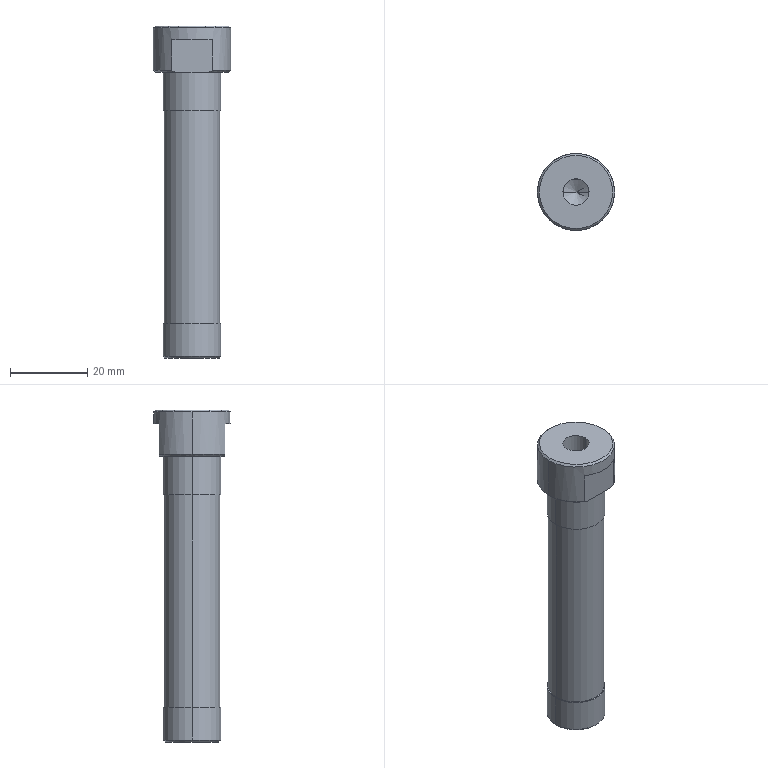Part | STEP file | 10000020474swp000-1 | 1 solid | 32 faces | box 20 x 20 x 86 mm | volume 15036 mm3 | cylinder 12 | cone 11 | plane 9 | commonest cylinder face diameters 15 x4 3.3 x2 6.8 x2 14.4 x2 20 x2
STEP:
#1=CARTESIAN_POINT('',(1.65,0.,-73.9));
#2=VERTEX_POINT('',#1);
#3=CARTESIAN_POINT('',(-1.65,0.,-73.9));
#4=VERTEX_POINT('',#3);
#5=CARTESIAN_POINT('',(0.,0.,-73.9));
#6=DIRECTION('',(0.,0.,-1.));
#7=DIRECTION('',(-1.,0.,0.));
#8=AXIS2_PLACEMENT_3D('',#5,#6,#7);
#9=CIRCLE('',#8,1.65);
#10=EDGE_CURVE('',#2,#4,#9,.T.);
#11=ORIENTED_EDGE('',*,*,#10,.F.);
#12=CARTESIAN_POINT('',(1.65,0.,-86.));
#13=VERTEX_POINT('',#12);
#14=CARTESIAN_POINT('',(1.65,0.,-86.));
#15=DIRECTION('',(0.,0.,-1.));
#16=VECTOR('',#15,1000.);
#17=LINE('',#14,#16);
#18=EDGE_CURVE('',#2,#13,#17,.T.);
#19=ORIENTED_EDGE('',*,*,#18,.T.);
#20=CARTESIAN_POINT('',(-1.65,0.,-86.));
#21=VERTEX_POINT('',#20);
#22=CARTESIAN_POINT('',(0.,0.,-86.));
#23=DIRECTION('',(0.,0.,-1.));
#24=DIRECTION('',(-1.,0.,0.));
#25=AXIS2_PLACEMENT_3D('',#22,#23,#24);
#26=CIRCLE('',#25,1.65);
#27=EDGE_CURVE('',#13,#21,#26,.T.);
#28=ORIENTED_EDGE('',*,*,#27,.T.);
#29=CARTESIAN_POINT('',(-1.65,0.,-86.));
#30=DIRECTION('',(0.,0.,-1.));
#31=VECTOR('',#30,1000.);
#32=LINE('',#29,#31);
#33=EDGE_CURVE('',#4,#21,#32,.T.);
#34=ORIENTED_EDGE('',*,*,#33,.F.);
#35=EDGE_LOOP('',(#11,#19,#28,#34));
#36=FACE_OUTER_BOUND('',#35,.T.);
#37=CARTESIAN_POINT('',(0.,0.,-86.));
#38=DIRECTION('',(0.,0.,-1.));
#39=DIRECTION('',(-1.,0.,0.));
#40=AXIS2_PLACEMENT_3D('',#37,#38,#39);
#41=CYLINDRICAL_SURFACE('',#40,1.65);
#42=ADVANCED_FACE('',(#36),#41,.F.);
#43=CARTESIAN_POINT('',(0.,0.,-72.909));
#44=VERTEX_POINT('',#43);
#45=CARTESIAN_POINT('',(-1.65,0.,-73.9));
#46=DIRECTION('',(-0.8572,0.,-0.515));
#47=VECTOR('',#46,1000.);
#48=LINE('',#45,#47);
#49=EDGE_CURVE('',#44,#4,#48,.T.);
#50=ORIENTED_EDGE('',*,*,#49,.F.);
#51=CARTESIAN_POINT('',(1.65,0.,-73.9));
#52=DIRECTION('',(0.8572,0.,-0.515));
#53=VECTOR('',#52,1000.);
#54=LINE('',#51,#53);
#55=EDGE_CURVE('',#44,#2,#54,.T.);
#56=ORIENTED_EDGE('',*,*,#55,.T.);
#57=ORIENTED_EDGE('',*,*,#10,.T.);
#58=EDGE_LOOP('',(#50,#56,#57));
#59=FACE_OUTER_BOUND('',#58,.T.);
#60=CARTESIAN_POINT('',(0.,0.,-73.9));
#61=DIRECTION('',(0.,0.,-1.));
#62=DIRECTION('',(-1.,0.,0.));
#63=AXIS2_PLACEMENT_3D('',#60,#61,#62);
#64=CONICAL_SURFACE('',#63,1.65,1.03);
#65=ADVANCED_FACE('',(#59),#64,.F.);
#66=CARTESIAN_POINT('',(9.5,0.,0.));
#67=VERTEX_POINT('',#66);
#68=CARTESIAN_POINT('',(-9.5,0.,0.));
#69=VERTEX_POINT('',#68);
#70=CARTESIAN_POINT('',(0.,0.,0.));
#71=DIRECTION('',(0.,0.,1.));
#72=DIRECTION('',(1.,0.,0.));
#73=AXIS2_PLACEMENT_3D('',#70,#71,#72);
#74=CIRCLE('',#73,9.5);
#75=EDGE_CURVE('',#67,#69,#74,.T.);
#76=ORIENTED_EDGE('',*,*,#75,.F.);
#77=CARTESIAN_POINT('',(10.,0.,-0.5));
#78=VERTEX_POINT('',#77);
#79=CARTESIAN_POINT('',(9.5,0.,0.));
#80=DIRECTION('',(0.7071,0.,-0.7071));
#81=VECTOR('',#80,1000.);
#82=LINE('',#79,#81);
#83=EDGE_CURVE('',#67,#78,#82,.T.);
#84=ORIENTED_EDGE('',*,*,#83,.T.);
#85=CARTESIAN_POINT('',(-10.,0.,-0.5));
#86=VERTEX_POINT('',#85);
#87=CARTESIAN_POINT('',(0.,0.,-0.5));
#88=DIRECTION('',(0.,0.,-1.));
#89=DIRECTION('',(1.,0.,0.));
#90=AXIS2_PLACEMENT_3D('',#87,#88,#89);
#91=CIRCLE('',#90,10.);
#92=EDGE_CURVE('',#86,#78,#91,.T.);
#93=ORIENTED_EDGE('',*,*,#92,.F.);
#94=CARTESIAN_POINT('',(-9.5,0.,0.));
#95=DIRECTION('',(-0.7071,0.,-0.7071));
#96=VECTOR('',#95,1000.);
#97=LINE('',#94,#96);
#98=EDGE_CURVE('',#69,#86,#97,.T.);
#99=ORIENTED_EDGE('',*,*,#98,.F.);
#100=EDGE_LOOP('',(#76,#84,#93,#99));
#101=FACE_OUTER_BOUND('',#100,.T.);
#102=CARTESIAN_POINT('',(0.,0.,0.));
#103=DIRECTION('',(0.,0.,-1.));
#104=DIRECTION('',(-1.,0.,0.));
#105=AXIS2_PLACEMENT_3D('',#102,#103,#104);
#106=CONICAL_SURFACE('',#105,9.5,0.7854);
#107=ADVANCED_FACE('',(#101),#106,.T.);
#108=CARTESIAN_POINT('',(-7.,0.,-86.));
#109=VERTEX_POINT('',#108);
#110=CARTESIAN_POINT('',(7.,0.,-86.));
#111=VERTEX_POINT('',#110);
#112=CARTESIAN_POINT('',(0.,0.,-86.));
#113=DIRECTION('',(0.,0.,-1.));
#114=DIRECTION('',(-1.,0.,0.));
#115=AXIS2_PLACEMENT_3D('',#112,#113,#114);
#116=CIRCLE('',#115,7.);
#117=EDGE_CURVE('',#109,#111,#116,.T.);
#118=ORIENTED_EDGE('',*,*,#117,.F.);
#119=CARTESIAN_POINT('',(-7.5,0.,-85.5));
#120=VERTEX_POINT('',#119);
#121=CARTESIAN_POINT('',(-7.,0.,-86.));
#122=DIRECTION('',(-0.7071,0.,0.7071));
#123=VECTOR('',#122,1000.);
#124=LINE('',#121,#123);
#125=EDGE_CURVE('',#109,#120,#124,.T.);
#126=ORIENTED_EDGE('',*,*,#125,.T.);
#127=CARTESIAN_POINT('',(7.5,0.,-85.5));
#128=VERTEX_POINT('',#127);
#129=CARTESIAN_POINT('',(0.,0.,-85.5));
#130=DIRECTION('',(0.,0.,1.));
#131=DIRECTION('',(-1.,0.,0.));
#132=AXIS2_PLACEMENT_3D('',#129,#130,#131);
#133=CIRCLE('',#132,7.5);
#134=EDGE_CURVE('',#128,#120,#133,.T.);
#135=ORIENTED_EDGE('',*,*,#134,.F.);
#136=CARTESIAN_POINT('',(7.,0.,-86.));
#137=DIRECTION('',(0.7071,0.,0.7071));
#138=VECTOR('',#137,1000.);
#139=LINE('',#136,#138);
#140=EDGE_CURVE('',#111,#128,#139,.T.);
#141=ORIENTED_EDGE('',*,*,#140,.F.);
#142=EDGE_LOOP('',(#118,#126,#135,#141));
#143=FACE_OUTER_BOUND('',#142,.T.);
#144=CARTESIAN_POINT('',(0.,0.,-86.));
#145=DIRECTION('',(0.,0.,1.));
#146=DIRECTION('',(1.,0.,0.));
#147=AXIS2_PLACEMENT_3D('',#144,#145,#146);
#148=CONICAL_SURFACE('',#147,7.,0.7854);
#149=ADVANCED_FACE('',(#143),#148,.T.);
#150=CARTESIAN_POINT('',(9.5,0.,-12.));
#151=VERTEX_POINT('',#150);
#152=CARTESIAN_POINT('',(4.243,-8.5,-12.));
#153=VERTEX_POINT('',#152);
#154=CARTESIAN_POINT('',(0.,0.,-12.));
#155=DIRECTION('',(0.,0.,-1.));
#156=DIRECTION('',(1.,0.,0.));
#157=AXIS2_PLACEMENT_3D('',#154,#155,#156);
#158=CIRCLE('',#157,9.5);
#159=EDGE_CURVE('',#151,#153,#158,.T.);
#160=ORIENTED_EDGE('',*,*,#159,.F.);
#161=CARTESIAN_POINT('',(10.,0.,-11.5));
#162=VERTEX_POINT('',#161);
#163=CARTESIAN_POINT('',(10.,0.,-11.5));
#164=DIRECTION('',(0.7071,0.,0.7071));
#165=VECTOR('',#164,1000.);
#166=LINE('',#163,#165);
#167=EDGE_CURVE('',#151,#162,#166,.T.);
#168=ORIENTED_EDGE('',*,*,#167,.T.);
#169=CARTESIAN_POINT('',(5.268,-8.5,-11.5));
#170=VERTEX_POINT('',#169);
#171=CARTESIAN_POINT('',(0.,0.,-11.5));
#172=DIRECTION('',(0.,0.,1.));
#173=DIRECTION('',(1.,0.,0.));
#174=AXIS2_PLACEMENT_3D('',#171,#172,#173);
#175=CIRCLE('',#174,10.);
#176=EDGE_CURVE('',#170,#162,#175,.T.);
#177=ORIENTED_EDGE('',*,*,#176,.F.);
#178=CARTESIAN_POINT('',(4.243,-8.5,-12.));
#179=CARTESIAN_POINT('',(4.59,-8.5,-11.845));
#180=CARTESIAN_POINT('',(4.931,-8.5,-11.677));
#181=CARTESIAN_POINT('',(5.268,-8.5,-11.5));
#182=B_SPLINE_CURVE_WITH_KNOTS('',3,(#178,#179,#180,#181),.UNSPECIFIED.,.F.,.F.,(4,4),(0.,0.001141),.UNSPECIFIED.);
#183=EDGE_CURVE('',#153,#170,#182,.T.);
#184=ORIENTED_EDGE('',*,*,#183,.F.);
#185=EDGE_LOOP('',(#160,#168,#177,#184));
#186=FACE_OUTER_BOUND('',#185,.T.);
#187=CARTESIAN_POINT('',(0.,0.,-11.5));
#188=DIRECTION('',(0.,0.,1.));
#189=DIRECTION('',(1.,0.,0.));
#190=AXIS2_PLACEMENT_3D('',#187,#188,#189);
#191=CONICAL_SURFACE('',#190,10.,0.7854);
#192=ADVANCED_FACE('',(#186),#191,.T.);
#193=CARTESIAN_POINT('',(-3.4,0.,-19.75));
#194=VERTEX_POINT('',#193);
#195=CARTESIAN_POINT('',(3.4,0.,-19.75));
#196=VERTEX_POINT('',#195);
#197=CARTESIAN_POINT('',(0.,0.,-19.75));
#198=DIRECTION('',(0.,0.,1.));
#199=DIRECTION('',(1.,0.,0.));
#200=AXIS2_PLACEMENT_3D('',#197,#198,#199);
#201=CIRCLE('',#200,3.4);
#202=EDGE_CURVE('',#194,#196,#201,.T.);
#203=ORIENTED_EDGE('',*,*,#202,.F.);
#204=CARTESIAN_POINT('',(-3.4,0.,0.));
#205=VERTEX_POINT('',#204);
#206=CARTESIAN_POINT('',(-3.4,0.,0.));
#207=DIRECTION('',(0.,0.,1.));
#208=VECTOR('',#207,1000.);
#209=LINE('',#206,#208);
#210=EDGE_CURVE('',#194,#205,#209,.T.);
#211=ORIENTED_EDGE('',*,*,#210,.T.);
#212=CARTESIAN_POINT('',(3.4,0.,0.));
#213=VERTEX_POINT('',#212);
#214=CARTESIAN_POINT('',(0.,0.,0.));
#215=DIRECTION('',(0.,0.,1.));
#216=DIRECTION('',(1.,0.,0.));
#217=AXIS2_PLACEMENT_3D('',#214,#215,#216);
#218=CIRCLE('',#217,3.4);
#219=EDGE_CURVE('',#205,#213,#218,.T.);
#220=ORIENTED_EDGE('',*,*,#219,.T.);
#221=CARTESIAN_POINT('',(3.4,0.,0.));
#222=DIRECTION('',(0.,0.,1.));
#223=VECTOR('',#222,1000.);
#224=LINE('',#221,#223);
#225=EDGE_CURVE('',#196,#213,#224,.T.);
#226=ORIENTED_EDGE('',*,*,#225,.F.);
#227=EDGE_LOOP('',(#203,#211,#220,#226));
#228=FACE_OUTER_BOUND('',#227,.T.);
#229=CARTESIAN_POINT('',(0.,0.,0.));
#230=DIRECTION('',(0.,0.,1.));
#231=DIRECTION('',(1.,0.,0.));
#232=AXIS2_PLACEMENT_3D('',#229,#230,#231);
#233=CYLINDRICAL_SURFACE('',#232,3.4);
#234=ADVANCED_FACE('',(#228),#233,.F.);
#235=CARTESIAN_POINT('',(0.,0.,-21.793));
#236=VERTEX_POINT('',#235);
#237=CARTESIAN_POINT('',(3.4,0.,-19.75));
#238=DIRECTION('',(0.8572,0.,0.515));
#239=VECTOR('',#238,1000.);
#240=LINE('',#237,#239);
#241=EDGE_CURVE('',#236,#196,#240,.T.);
#242=ORIENTED_EDGE('',*,*,#241,.F.);
#243=CARTESIAN_POINT('',(-3.4,0.,-19.75));
#244=DIRECTION('',(-0.8572,0.,0.515));
#245=VECTOR('',#244,1000.);
#246=LINE('',#243,#245);
#247=EDGE_CURVE('',#236,#194,#246,.T.);
#248=ORIENTED_EDGE('',*,*,#247,.T.);
#249=ORIENTED_EDGE('',*,*,#202,.T.);
#250=EDGE_LOOP('',(#242,#248,#249));
#251=FACE_OUTER_BOUND('',#250,.T.);
#252=CARTESIAN_POINT('',(0.,0.,-19.75));
#253=DIRECTION('',(0.,0.,1.));
#254=DIRECTION('',(1.,0.,0.));
#255=AXIS2_PLACEMENT_3D('',#252,#253,#254);
#256=CONICAL_SURFACE('',#255,3.4,1.03);
#257=ADVANCED_FACE('',(#251),#256,.F.);
#258=ORIENTED_EDGE('',*,*,#134,.T.);
#259=CARTESIAN_POINT('',(-7.5,0.,-77.));
#260=VERTEX_POINT('',#259);
#261=CARTESIAN_POINT('',(-7.5,0.,-86.));
#262=DIRECTION('',(0.,0.,1.));
#263=VECTOR('',#262,1000.);
#264=LINE('',#261,#263);
#265=EDGE_CURVE('',#120,#260,#264,.T.);
#266=ORIENTED_EDGE('',*,*,#265,.T.);
#267=CARTESIAN_POINT('',(7.5,0.,-77.));
#268=VERTEX_POINT('',#267);
#269=CARTESIAN_POINT('',(0.,0.,-77.));
#270=DIRECTION('',(0.,0.,-1.));
#271=DIRECTION('',(-1.,0.,0.));
#272=AXIS2_PLACEMENT_3D('',#269,#270,#271);
#273=CIRCLE('',#272,7.5);
#274=EDGE_CURVE('',#260,#268,#273,.T.);
#275=ORIENTED_EDGE('',*,*,#274,.T.);
#276=CARTESIAN_POINT('',(7.5,0.,-86.));
#277=DIRECTION('',(0.,0.,1.));
#278=VECTOR('',#277,1000.);
#279=LINE('',#276,#278);
#280=EDGE_CURVE('',#128,#268,#279,.T.);
#281=ORIENTED_EDGE('',*,*,#280,.F.);
#282=EDGE_LOOP('',(#258,#266,#275,#281));
#283=FACE_OUTER_BOUND('',#282,.T.);
#284=CARTESIAN_POINT('',(0.,0.,-86.));
#285=DIRECTION('',(0.,0.,1.));
#286=DIRECTION('',(1.,0.,0.));
#287=AXIS2_PLACEMENT_3D('',#284,#285,#286);
#288=CYLINDRICAL_SURFACE('',#287,7.5);
#289=ADVANCED_FACE('',(#283),#288,.T.);
#290=CARTESIAN_POINT('',(-7.2,0.,-77.));
#291=VERTEX_POINT('',#290);
#292=CARTESIAN_POINT('',(7.2,0.,-77.));
#293=VERTEX_POINT('',#292);
#294=CARTESIAN_POINT('',(0.,0.,-77.));
#295=DIRECTION('',(0.,0.,-1.));
#296=DIRECTION('',(-1.,0.,0.));
#297=AXIS2_PLACEMENT_3D('',#294,#295,#296);
#298=CIRCLE('',#297,7.2);
#299=EDGE_CURVE('',#291,#293,#298,.T.);
#300=ORIENTED_EDGE('',*,*,#299,.F.);
#301=CARTESIAN_POINT('',(-7.2,0.,-22.));
#302=VERTEX_POINT('',#301);
#303=CARTESIAN_POINT('',(-7.2,0.,-77.));
#304=DIRECTION('',(0.,0.,1.));
#305=VECTOR('',#304,1000.);
#306=LINE('',#303,#305);
#307=EDGE_CURVE('',#291,#302,#306,.T.);
#308=ORIENTED_EDGE('',*,*,#307,.T.);
#309=CARTESIAN_POINT('',(7.2,0.,-22.));
#310=VERTEX_POINT('',#309);
#311=CARTESIAN_POINT('',(0.,0.,-22.));
#312=DIRECTION('',(0.,0.,-1.));
#313=DIRECTION('',(-1.,0.,0.));
#314=AXIS2_PLACEMENT_3D('',#311,#312,#313);
#315=CIRCLE('',#314,7.2);
#316=EDGE_CURVE('',#302,#310,#315,.T.);
#317=ORIENTED_EDGE('',*,*,#316,.T.);
#318=CARTESIAN_POINT('',(7.2,0.,-77.));
#319=DIRECTION('',(0.,0.,1.));
#320=VECTOR('',#319,1000.);
#321=LINE('',#318,#320);
#322=EDGE_CURVE('',#293,#310,#321,.T.);
#323=ORIENTED_EDGE('',*,*,#322,.F.);
#324=EDGE_LOOP('',(#300,#308,#317,#323));
#325=FACE_OUTER_BOUND('',#324,.T.);
#326=CARTESIAN_POINT('',(0.,0.,-77.));
#327=DIRECTION('',(0.,0.,1.));
#328=DIRECTION('',(1.,0.,0.));
#329=AXIS2_PLACEMENT_3D('',#326,#327,#328);
#330=CYLINDRICAL_SURFACE('',#329,7.2);
#331=ADVANCED_FACE('',(#325),#330,.T.);
#332=CARTESIAN_POINT('',(-7.5,0.,-22.));
#333=VERTEX_POINT('',#332);
#334=CARTESIAN_POINT('',(7.5,0.,-22.));
#335=VERTEX_POINT('',#334);
#336=CARTESIAN_POINT('',(0.,0.,-22.));
#337=DIRECTION('',(0.,0.,-1.));
#338=DIRECTION('',(-1.,0.,0.));
#339=AXIS2_PLACEMENT_3D('',#336,#337,#338);
#340=CIRCLE('',#339,7.5);
#341=EDGE_CURVE('',#333,#335,#340,.T.);
#342=ORIENTED_EDGE('',*,*,#341,.F.);
#343=CARTESIAN_POINT('',(-7.5,0.,-12.));
#344=VERTEX_POINT('',#343);
#345=CARTESIAN_POINT('',(-7.5,0.,-22.));
#346=DIRECTION('',(0.,0.,1.));
#347=VECTOR('',#346,1000.);
#348=LINE('',#345,#347);
#349=EDGE_CURVE('',#333,#344,#348,.T.);
#350=ORIENTED_EDGE('',*,*,#349,.T.);
#351=CARTESIAN_POINT('',(7.5,0.,-12.));
#352=VERTEX_POINT('',#351);
#353=CARTESIAN_POINT('',(0.,0.,-12.));
#354=DIRECTION('',(0.,0.,-1.));
#355=DIRECTION('',(1.,0.,0.));
#356=AXIS2_PLACEMENT_3D('',#353,#354,#355);
#357=CIRCLE('',#356,7.5);
#358=EDGE_CURVE('',#344,#352,#357,.T.);
#359=ORIENTED_EDGE('',*,*,#358,.T.);
#360=CARTESIAN_POINT('',(7.5,0.,-22.));
#361=DIRECTION('',(0.,0.,1.));
#362=VECTOR('',#361,1000.);
#363=LINE('',#360,#362);
#364=EDGE_CURVE('',#335,#352,#363,.T.);
#365=ORIENTED_EDGE('',*,*,#364,.F.);
#366=EDGE_LOOP('',(#342,#350,#359,#365));
#367=FACE_OUTER_BOUND('',#366,.T.);
#368=CARTESIAN_POINT('',(0.,0.,-22.));
#369=DIRECTION('',(0.,0.,1.));
#370=DIRECTION('',(1.,0.,0.));
#371=AXIS2_PLACEMENT_3D('',#368,#369,#370);
#372=CYLINDRICAL_SURFACE('',#371,7.5);
#373=ADVANCED_FACE('',(#367),#372,.T.);
#374=CARTESIAN_POINT('',(-5.268,8.5,-11.5));
#375=VERTEX_POINT('',#374);
#376=CARTESIAN_POINT('',(-10.,0.,-11.5));
#377=VERTEX_POINT('',#376);
#378=CARTESIAN_POINT('',(0.,0.,-11.5));
#379=DIRECTION('',(0.,0.,1.));
#380=DIRECTION('',(1.,0.,0.));
#381=AXIS2_PLACEMENT_3D('',#378,#379,#380);
#382=CIRCLE('',#381,10.);
#383=EDGE_CURVE('',#375,#377,#382,.T.);
#384=ORIENTED_EDGE('',*,*,#383,.T.);
#385=CARTESIAN_POINT('',(-10.,0.,-12.));
#386=DIRECTION('',(0.,0.,1.));
#387=VECTOR('',#386,1000.);
#388=LINE('',#385,#387);
#389=EDGE_CURVE('',#377,#86,#388,.T.);
#390=ORIENTED_EDGE('',*,*,#389,.T.);
#391=ORIENTED_EDGE('',*,*,#92,.T.);
#392=CARTESIAN_POINT('',(10.,0.,-12.));
#393=DIRECTION('',(0.,0.,1.));
#394=VECTOR('',#393,1000.);
#395=LINE('',#392,#394);
#396=EDGE_CURVE('',#162,#78,#395,.T.);
#397=ORIENTED_EDGE('',*,*,#396,.F.);
#398=CARTESIAN_POINT('',(5.268,8.5,-11.5));
#399=VERTEX_POINT('',#398);
#400=CARTESIAN_POINT('',(0.,0.,-11.5));
#401=DIRECTION('',(0.,0.,1.));
#402=DIRECTION('',(1.,0.,0.));
#403=AXIS2_PLACEMENT_3D('',#400,#401,#402);
#404=CIRCLE('',#403,10.);
#405=EDGE_CURVE('',#162,#399,#404,.T.);
#406=ORIENTED_EDGE('',*,*,#405,.T.);
#407=CARTESIAN_POINT('',(5.268,8.5,-3.5));
#408=VERTEX_POINT('',#407);
#409=CARTESIAN_POINT('',(5.268,8.5,-12.));
#410=DIRECTION('',(0.,0.,1.));
#411=VECTOR('',#410,1000.);
#412=LINE('',#409,#411);
#413=EDGE_CURVE('',#399,#408,#412,.T.);
#414=ORIENTED_EDGE('',*,*,#413,.T.);
#415=CARTESIAN_POINT('',(-5.268,8.5,-3.5));
#416=VERTEX_POINT('',#415);
#417=CARTESIAN_POINT('',(0.,0.,-3.5));
#418=DIRECTION('',(0.,0.,1.));
#419=DIRECTION('',(-1.,0.,0.));
#420=AXIS2_PLACEMENT_3D('',#417,#418,#419);
#421=CIRCLE('',#420,10.);
#422=EDGE_CURVE('',#408,#416,#421,.T.);
#423=ORIENTED_EDGE('',*,*,#422,.T.);
#424=CARTESIAN_POINT('',(-5.268,8.5,-12.));
#425=DIRECTION('',(0.,0.,-1.));
#426=VECTOR('',#425,1000.);
#427=LINE('',#424,#426);
#428=EDGE_CURVE('',#416,#375,#427,.T.);
#429=ORIENTED_EDGE('',*,*,#428,.T.);
#430=EDGE_LOOP('',(#384,#390,#391,#397,#406,#414,#423,#429));
#431=FACE_OUTER_BOUND('',#430,.T.);
#432=CARTESIAN_POINT('',(0.,0.,-12.));
#433=DIRECTION('',(0.,0.,1.));
#434=DIRECTION('',(1.,0.,0.));
#435=AXIS2_PLACEMENT_3D('',#432,#433,#434);
#436=CYLINDRICAL_SURFACE('',#435,10.);
#437=ADVANCED_FACE('',(#431),#436,.T.);
#438=ORIENTED_EDGE('',*,*,#389,.F.);
#439=CARTESIAN_POINT('',(-5.268,-8.5,-11.5));
#440=VERTEX_POINT('',#439);
#441=CARTESIAN_POINT('',(0.,0.,-11.5));
#442=DIRECTION('',(0.,0.,1.));
#443=DIRECTION('',(1.,0.,0.));
#444=AXIS2_PLACEMENT_3D('',#441,#442,#443);
#445=CIRCLE('',#444,10.);
#446=EDGE_CURVE('',#377,#440,#445,.T.);
#447=ORIENTED_EDGE('',*,*,#446,.T.);
#448=CARTESIAN_POINT('',(-5.268,-8.5,-3.5));
#449=VERTEX_POINT('',#448);
#450=CARTESIAN_POINT('',(-5.268,-8.5,-12.));
#451=DIRECTION('',(0.,0.,1.));
#452=VECTOR('',#451,1000.);
#453=LINE('',#450,#452);
#454=EDGE_CURVE('',#440,#449,#453,.T.);
#455=ORIENTED_EDGE('',*,*,#454,.T.);
#456=CARTESIAN_POINT('',(5.268,-8.5,-3.5));
#457=VERTEX_POINT('',#456);
#458=CARTESIAN_POINT('',(0.,0.,-3.5));
#459=DIRECTION('',(0.,0.,-1.));
#460=DIRECTION('',(1.,0.,0.));
#461=AXIS2_PLACEMENT_3D('',#458,#459,#460);
#462=CIRCLE('',#461,10.);
#463=EDGE_CURVE('',#457,#449,#462,.T.);
#464=ORIENTED_EDGE('',*,*,#463,.F.);
#465=CARTESIAN_POINT('',(5.268,-8.5,-12.));
#466=DIRECTION('',(0.,0.,-1.));
#467=VECTOR('',#466,1000.);
#468=LINE('',#465,#467);
#469=EDGE_CURVE('',#457,#170,#468,.T.);
#470=ORIENTED_EDGE('',*,*,#469,.T.);
#471=ORIENTED_EDGE('',*,*,#176,.T.);
#472=ORIENTED_EDGE('',*,*,#396,.T.);
#473=CARTESIAN_POINT('',(0.,0.,-0.5));
#474=DIRECTION('',(0.,0.,-1.));
#475=DIRECTION('',(1.,0.,0.));
#476=AXIS2_PLACEMENT_3D('',#473,#474,#475);
#477=CIRCLE('',#476,10.);
#478=EDGE_CURVE('',#78,#86,#477,.T.);
#479=ORIENTED_EDGE('',*,*,#478,.T.);
#480=EDGE_LOOP('',(#438,#447,#455,#464,#470,#471,#472,#479));
#481=FACE_OUTER_BOUND('',#480,.T.);
#482=CARTESIAN_POINT('',(0.,0.,-12.));
#483=DIRECTION('',(0.,0.,1.));
#484=DIRECTION('',(1.,0.,0.));
#485=AXIS2_PLACEMENT_3D('',#482,#483,#484);
#486=CYLINDRICAL_SURFACE('',#485,10.);
#487=ADVANCED_FACE('',(#481),#486,.T.);
#488=CARTESIAN_POINT('',(0.,0.,-12.));
#489=DIRECTION('',(0.,0.,-1.));
#490=DIRECTION('',(1.,0.,0.));
#491=AXIS2_PLACEMENT_3D('',#488,#489,#490);
#492=CIRCLE('',#491,7.5);
#493=EDGE_CURVE('',#352,#344,#492,.T.);
#494=ORIENTED_EDGE('',*,*,#493,.F.);
#495=ORIENTED_EDGE('',*,*,#358,.F.);
#496=EDGE_LOOP('',(#494,#495));
#497=FACE_BOUND('',#496,.T.);
#498=CARTESIAN_POINT('',(4.243,8.5,-12.));
#499=VERTEX_POINT('',#498);
#500=CARTESIAN_POINT('',(-4.243,8.5,-12.));
#501=VERTEX_POINT('',#500);
#502=CARTESIAN_POINT('',(0.,8.5,-12.));
#503=DIRECTION('',(-1.,0.,0.));
#504=VECTOR('',#503,1000.);
#505=LINE('',#502,#504);
#506=EDGE_CURVE('',#499,#501,#505,.T.);
#507=ORIENTED_EDGE('',*,*,#506,.F.);
#508=CARTESIAN_POINT('',(0.,0.,-12.));
#509=DIRECTION('',(0.,0.,-1.));
#510=DIRECTION('',(1.,0.,0.));
#511=AXIS2_PLACEMENT_3D('',#508,#509,#510);
#512=CIRCLE('',#511,9.5);
#513=EDGE_CURVE('',#499,#151,#512,.T.);
#514=ORIENTED_EDGE('',*,*,#513,.T.);
#515=ORIENTED_EDGE('',*,*,#159,.T.);
#516=CARTESIAN_POINT('',(-4.243,-8.5,-12.));
#517=VERTEX_POINT('',#516);
#518=CARTESIAN_POINT('',(0.,-8.5,-12.));
#519=DIRECTION('',(1.,0.,0.));
#520=VECTOR('',#519,1000.);
#521=LINE('',#518,#520);
#522=EDGE_CURVE('',#517,#153,#521,.T.);
#523=ORIENTED_EDGE('',*,*,#522,.F.);
#524=CARTESIAN_POINT('',(0.,0.,-12.));
#525=DIRECTION('',(0.,0.,-1.));
#526=DIRECTION('',(1.,0.,0.));
#527=AXIS2_PLACEMENT_3D('',#524,#525,#526);
#528=CIRCLE('',#527,9.5);
#529=EDGE_CURVE('',#517,#501,#528,.T.);
#530=ORIENTED_EDGE('',*,*,#529,.T.);
#531=EDGE_LOOP('',(#507,#514,#515,#523,#530));
#532=FACE_OUTER_BOUND('',#531,.T.);
#533=CARTESIAN_POINT('',(0.,0.,-12.));
#534=DIRECTION('',(0.,0.,1.));
#535=DIRECTION('',(1.,0.,0.));
#536=AXIS2_PLACEMENT_3D('',#533,#534,#535);
#537=PLANE('',#536);
#538=ADVANCED_FACE('',(#497,#532),#537,.F.);
#539=CARTESIAN_POINT('',(0.,0.,0.));
#540=DIRECTION('',(0.,0.,1.));
#541=DIRECTION('',(1.,0.,0.));
#542=AXIS2_PLACEMENT_3D('',#539,#540,#541);
#543=CIRCLE('',#542,9.5);
#544=EDGE_CURVE('',#69,#67,#543,.T.);
#545=ORIENTED_EDGE('',*,*,#544,.T.);
#546=ORIENTED_EDGE('',*,*,#75,.T.);
#547=EDGE_LOOP('',(#545,#546));
#548=FACE_OUTER_BOUND('',#547,.T.);
#549=CARTESIAN_POINT('',(0.,0.,0.));
#550=DIRECTION('',(0.,0.,1.));
#551=DIRECTION('',(1.,0.,0.));
#552=AXIS2_PLACEMENT_3D('',#549,#550,#551);
#553=CIRCLE('',#552,3.4);
#554=EDGE_CURVE('',#213,#205,#553,.T.);
#555=ORIENTED_EDGE('',*,*,#554,.F.);
#556=ORIENTED_EDGE('',*,*,#219,.F.);
#557=EDGE_LOOP('',(#555,#556));
#558=FACE_BOUND('',#557,.T.);
#559=CARTESIAN_POINT('',(0.,0.,0.));
#560=DIRECTION('',(0.,0.,1.));
#561=DIRECTION('',(1.,0.,0.));
#562=AXIS2_PLACEMENT_3D('',#559,#560,#561);
#563=PLANE('',#562);
#564=ADVANCED_FACE('',(#548,#558),#563,.T.);
#565=ORIENTED_EDGE('',*,*,#349,.F.);
#566=CARTESIAN_POINT('',(0.,0.,-22.));
#567=DIRECTION('',(0.,0.,-1.));
#568=DIRECTION('',(-1.,0.,0.));
#569=AXIS2_PLACEMENT_3D('',#566,#567,#568);
#570=CIRCLE('',#569,7.5);
#571=EDGE_CURVE('',#335,#333,#570,.T.);
#572=ORIENTED_EDGE('',*,*,#571,.F.);
#573=ORIENTED_EDGE('',*,*,#364,.T.);
#574=ORIENTED_EDGE('',*,*,#493,.T.);
#575=EDGE_LOOP('',(#565,#572,#573,#574));
#576=FACE_OUTER_BOUND('',#575,.T.);
#577=CARTESIAN_POINT('',(0.,0.,-22.));
#578=DIRECTION('',(0.,0.,1.));
#579=DIRECTION('',(1.,0.,0.));
#580=AXIS2_PLACEMENT_3D('',#577,#578,#579);
#581=CYLINDRICAL_SURFACE('',#580,7.5);
#582=ADVANCED_FACE('',(#576),#581,.T.);
#583=CARTESIAN_POINT('',(0.,0.,-22.));
#584=DIRECTION('',(0.,0.,-1.));
#585=DIRECTION('',(-1.,0.,0.));
#586=AXIS2_PLACEMENT_3D('',#583,#584,#585);
#587=CIRCLE('',#586,7.2);
#588=EDGE_CURVE('',#310,#302,#587,.T.);
#589=ORIENTED_EDGE('',*,*,#588,.F.);
#590=ORIENTED_EDGE('',*,*,#316,.F.);
#591=EDGE_LOOP('',(#589,#590));
#592=FACE_BOUND('',#591,.T.);
#593=ORIENTED_EDGE('',*,*,#571,.T.);
#594=ORIENTED_EDGE('',*,*,#341,.T.);
#595=EDGE_LOOP('',(#593,#594));
#596=FACE_OUTER_BOUND('',#595,.T.);
#597=CARTESIAN_POINT('',(0.,0.,-22.));
#598=DIRECTION('',(0.,0.,-1.));
#599=DIRECTION('',(-1.,0.,0.));
#600=AXIS2_PLACEMENT_3D('',#597,#598,#599);
#601=PLANE('',#600);
#602=ADVANCED_FACE('',(#592,#596),#601,.T.);
#603=ORIENTED_EDGE('',*,*,#307,.F.);
#604=CARTESIAN_POINT('',(0.,0.,-77.));
#605=DIRECTION('',(0.,0.,-1.));
#606=DIRECTION('',(-1.,0.,0.));
#607=AXIS2_PLACEMENT_3D('',#604,#605,#606);
#608=CIRCLE('',#607,7.2);
#609=EDGE_CURVE('',#293,#291,#608,.T.);
#610=ORIENTED_EDGE('',*,*,#609,.F.);
#611=ORIENTED_EDGE('',*,*,#322,.T.);
#612=ORIENTED_EDGE('',*,*,#588,.T.);
#613=EDGE_LOOP('',(#603,#610,#611,#612));
#614=FACE_OUTER_BOUND('',#613,.T.);
#615=CARTESIAN_POINT('',(0.,0.,-77.));
#616=DIRECTION('',(0.,0.,1.));
#617=DIRECTION('',(1.,0.,0.));
#618=AXIS2_PLACEMENT_3D('',#615,#616,#617);
#619=CYLINDRICAL_SURFACE('',#618,7.2);
#620=ADVANCED_FACE('',(#614),#619,.T.);
#621=ORIENTED_EDGE('',*,*,#265,.F.);
#622=CARTESIAN_POINT('',(0.,0.,-85.5));
#623=DIRECTION('',(0.,0.,1.));
#624=DIRECTION('',(-1.,0.,0.));
#625=AXIS2_PLACEMENT_3D('',#622,#623,#624);
#626=CIRCLE('',#625,7.5);
#627=EDGE_CURVE('',#120,#128,#626,.T.);
#628=ORIENTED_EDGE('',*,*,#627,.T.);
#629=ORIENTED_EDGE('',*,*,#280,.T.);
#630=CARTESIAN_POINT('',(0.,0.,-77.));
#631=DIRECTION('',(0.,0.,-1.));
#632=DIRECTION('',(-1.,0.,0.));
#633=AXIS2_PLACEMENT_3D('',#630,#631,#632);
#634=CIRCLE('',#633,7.5);
#635=EDGE_CURVE('',#268,#260,#634,.T.);
#636=ORIENTED_EDGE('',*,*,#635,.T.);
#637=EDGE_LOOP('',(#621,#628,#629,#636));
#638=FACE_OUTER_BOUND('',#637,.T.);
#639=CARTESIAN_POINT('',(0.,0.,-86.));
#640=DIRECTION('',(0.,0.,1.));
#641=DIRECTION('',(1.,0.,0.));
#642=AXIS2_PLACEMENT_3D('',#639,#640,#641);
#643=CYLINDRICAL_SURFACE('',#642,7.5);
#644=ADVANCED_FACE('',(#638),#643,.T.);
#645=CARTESIAN_POINT('',(0.,0.,-86.));
#646=DIRECTION('',(0.,0.,-1.));
#647=DIRECTION('',(-1.,0.,0.));
#648=AXIS2_PLACEMENT_3D('',#645,#646,#647);
#649=CIRCLE('',#648,1.65);
#650=EDGE_CURVE('',#21,#13,#649,.T.);
#651=ORIENTED_EDGE('',*,*,#650,.F.);
#652=ORIENTED_EDGE('',*,*,#27,.F.);
#653=EDGE_LOOP('',(#651,#652));
#654=FACE_BOUND('',#653,.T.);
#655=CARTESIAN_POINT('',(0.,0.,-86.));
#656=DIRECTION('',(0.,0.,-1.));
#657=DIRECTION('',(-1.,0.,0.));
#658=AXIS2_PLACEMENT_3D('',#655,#656,#657);
#659=CIRCLE('',#658,7.);
#660=EDGE_CURVE('',#111,#109,#659,.T.);
#661=ORIENTED_EDGE('',*,*,#660,.T.);
#662=ORIENTED_EDGE('',*,*,#117,.T.);
#663=EDGE_LOOP('',(#661,#662));
#664=FACE_OUTER_BOUND('',#663,.T.);
#665=CARTESIAN_POINT('',(0.,0.,-86.));
#666=DIRECTION('',(0.,0.,-1.));
#667=DIRECTION('',(-1.,0.,0.));
#668=AXIS2_PLACEMENT_3D('',#665,#666,#667);
#669=PLANE('',#668);
#670=ADVANCED_FACE('',(#654,#664),#669,.T.);
#671=ORIENTED_EDGE('',*,*,#609,.T.);
#672=ORIENTED_EDGE('',*,*,#299,.T.);
#673=EDGE_LOOP('',(#671,#672));
#674=FACE_BOUND('',#673,.T.);
#675=ORIENTED_EDGE('',*,*,#635,.F.);
#676=ORIENTED_EDGE('',*,*,#274,.F.);
#677=EDGE_LOOP('',(#675,#676));
#678=FACE_OUTER_BOUND('',#677,.T.);
#679=CARTESIAN_POINT('',(0.,0.,-77.));
#680=DIRECTION('',(0.,0.,-1.));
#681=DIRECTION('',(-1.,0.,0.));
#682=AXIS2_PLACEMENT_3D('',#679,#680,#681);
#683=PLANE('',#682);
#684=ADVANCED_FACE('',(#674,#678),#683,.F.);
#685=ORIENTED_EDGE('',*,*,#247,.F.);
#686=ORIENTED_EDGE('',*,*,#241,.T.);
#687=CARTESIAN_POINT('',(0.,0.,-19.75));
#688=DIRECTION('',(0.,0.,1.));
#689=DIRECTION('',(1.,0.,0.));
#690=AXIS2_PLACEMENT_3D('',#687,#688,#689);
#691=CIRCLE('',#690,3.4);
#692=EDGE_CURVE('',#196,#194,#691,.T.);
#693=ORIENTED_EDGE('',*,*,#692,.T.);
#694=EDGE_LOOP('',(#685,#686,#693));
#695=FACE_OUTER_BOUND('',#694,.T.);
#696=CARTESIAN_POINT('',(0.,0.,-19.75));
#697=DIRECTION('',(0.,0.,1.));
#698=DIRECTION('',(1.,0.,0.));
#699=AXIS2_PLACEMENT_3D('',#696,#697,#698);
#700=CONICAL_SURFACE('',#699,3.4,1.03);
#701=ADVANCED_FACE('',(#695),#700,.F.);
#702=ORIENTED_EDGE('',*,*,#210,.F.);
#703=ORIENTED_EDGE('',*,*,#692,.F.);
#704=ORIENTED_EDGE('',*,*,#225,.T.);
#705=ORIENTED_EDGE('',*,*,#554,.T.);
#706=EDGE_LOOP('',(#702,#703,#704,#705));
#707=FACE_OUTER_BOUND('',#706,.T.);
#708=CARTESIAN_POINT('',(0.,0.,0.));
#709=DIRECTION('',(0.,0.,1.));
#710=DIRECTION('',(1.,0.,0.));
#711=AXIS2_PLACEMENT_3D('',#708,#709,#710);
#712=CYLINDRICAL_SURFACE('',#711,3.4);
#713=ADVANCED_FACE('',(#707),#712,.F.);
#714=CARTESIAN_POINT('',(-10.,8.5,-3.5));
#715=DIRECTION('',(1.,0.,0.));
#716=VECTOR('',#715,1000.);
#717=LINE('',#714,#716);
#718=EDGE_CURVE('',#416,#408,#717,.T.);
#719=ORIENTED_EDGE('',*,*,#718,.F.);
#720=ORIENTED_EDGE('',*,*,#422,.F.);
#721=EDGE_LOOP('',(#719,#720));
#722=FACE_OUTER_BOUND('',#721,.T.);
#723=CARTESIAN_POINT('',(-10.,10.,-3.5));
#724=DIRECTION('',(0.,0.,-1.));
#725=DIRECTION('',(-1.,0.,0.));
#726=AXIS2_PLACEMENT_3D('',#723,#724,#725);
#727=PLANE('',#726);
#728=ADVANCED_FACE('',(#722),#727,.T.);
#729=ORIENTED_EDGE('',*,*,#413,.F.);
#730=CARTESIAN_POINT('',(5.268,8.5,-11.5));
#731=CARTESIAN_POINT('',(4.931,8.5,-11.677));
#732=CARTESIAN_POINT('',(4.59,8.5,-11.845));
#733=CARTESIAN_POINT('',(4.243,8.5,-12.));
#734=B_SPLINE_CURVE_WITH_KNOTS('',3,(#730,#731,#732,#733),.UNSPECIFIED.,.F.,.F.,(4,4),(0.,0.001141),.UNSPECIFIED.);
#735=EDGE_CURVE('',#399,#499,#734,.T.);
#736=ORIENTED_EDGE('',*,*,#735,.T.);
#737=ORIENTED_EDGE('',*,*,#506,.T.);
#738=CARTESIAN_POINT('',(-4.243,8.5,-12.));
#739=CARTESIAN_POINT('',(-4.59,8.5,-11.845));
#740=CARTESIAN_POINT('',(-4.931,8.5,-11.677));
#741=CARTESIAN_POINT('',(-5.268,8.5,-11.5));
#742=B_SPLINE_CURVE_WITH_KNOTS('',3,(#738,#739,#740,#741),.UNSPECIFIED.,.F.,.F.,(4,4),(0.,0.001141),.UNSPECIFIED.);
#743=EDGE_CURVE('',#501,#375,#742,.T.);
#744=ORIENTED_EDGE('',*,*,#743,.T.);
#745=ORIENTED_EDGE('',*,*,#428,.F.);
#746=ORIENTED_EDGE('',*,*,#718,.T.);
#747=EDGE_LOOP('',(#729,#736,#737,#744,#745,#746));
#748=FACE_OUTER_BOUND('',#747,.T.);
#749=CARTESIAN_POINT('',(0.,8.5,0.));
#750=DIRECTION('',(0.,1.,0.));
#751=DIRECTION('',(0.,0.,1.));
#752=AXIS2_PLACEMENT_3D('',#749,#750,#751);
#753=PLANE('',#752);
#754=ADVANCED_FACE('',(#748),#753,.T.);
#755=CARTESIAN_POINT('',(-10.,-8.5,-3.5));
#756=DIRECTION('',(1.,0.,0.));
#757=VECTOR('',#756,1000.);
#758=LINE('',#755,#757);
#759=EDGE_CURVE('',#449,#457,#758,.T.);
#760=ORIENTED_EDGE('',*,*,#759,.T.);
#761=ORIENTED_EDGE('',*,*,#463,.T.);
#762=EDGE_LOOP('',(#760,#761));
#763=FACE_OUTER_BOUND('',#762,.T.);
#764=CARTESIAN_POINT('',(-10.,-10.,-3.5));
#765=DIRECTION('',(0.,0.,1.));
#766=DIRECTION('',(1.,0.,0.));
#767=AXIS2_PLACEMENT_3D('',#764,#765,#766);
#768=PLANE('',#767);
#769=ADVANCED_FACE('',(#763),#768,.F.);
#770=ORIENTED_EDGE('',*,*,#522,.T.);
#771=ORIENTED_EDGE('',*,*,#183,.T.);
#772=ORIENTED_EDGE('',*,*,#469,.F.);
#773=ORIENTED_EDGE('',*,*,#759,.F.);
#774=ORIENTED_EDGE('',*,*,#454,.F.);
#775=CARTESIAN_POINT('',(-5.268,-8.5,-11.5));
#776=CARTESIAN_POINT('',(-4.931,-8.5,-11.677));
#777=CARTESIAN_POINT('',(-4.59,-8.5,-11.845));
#778=CARTESIAN_POINT('',(-4.243,-8.5,-12.));
#779=B_SPLINE_CURVE_WITH_KNOTS('',3,(#775,#776,#777,#778),.UNSPECIFIED.,.F.,.F.,(4,4),(0.,0.001141),.UNSPECIFIED.);
#780=EDGE_CURVE('',#440,#517,#779,.T.);
#781=ORIENTED_EDGE('',*,*,#780,.T.);
#782=EDGE_LOOP('',(#770,#771,#772,#773,#774,#781));
#783=FACE_OUTER_BOUND('',#782,.T.);
#784=CARTESIAN_POINT('',(0.,-8.5,0.));
#785=DIRECTION('',(0.,-1.,0.));
#786=DIRECTION('',(0.,0.,1.));
#787=AXIS2_PLACEMENT_3D('',#784,#785,#786);
#788=PLANE('',#787);
#789=ADVANCED_FACE('',(#783),#788,.T.);
#790=ORIENTED_EDGE('',*,*,#167,.F.);
#791=ORIENTED_EDGE('',*,*,#513,.F.);
#792=ORIENTED_EDGE('',*,*,#735,.F.);
#793=ORIENTED_EDGE('',*,*,#405,.F.);
#794=EDGE_LOOP('',(#790,#791,#792,#793));
#795=FACE_OUTER_BOUND('',#794,.T.);
#796=CARTESIAN_POINT('',(0.,0.,-11.5));
#797=DIRECTION('',(0.,0.,1.));
#798=DIRECTION('',(1.,0.,0.));
#799=AXIS2_PLACEMENT_3D('',#796,#797,#798);
#800=CONICAL_SURFACE('',#799,10.,0.7854);
#801=ADVANCED_FACE('',(#795),#800,.T.);
#802=ORIENTED_EDGE('',*,*,#743,.F.);
#803=ORIENTED_EDGE('',*,*,#529,.F.);
#804=ORIENTED_EDGE('',*,*,#780,.F.);
#805=ORIENTED_EDGE('',*,*,#446,.F.);
#806=ORIENTED_EDGE('',*,*,#383,.F.);
#807=EDGE_LOOP('',(#802,#803,#804,#805,#806));
#808=FACE_OUTER_BOUND('',#807,.T.);
#809=CARTESIAN_POINT('',(0.,0.,-11.5));
#810=DIRECTION('',(0.,0.,1.));
#811=DIRECTION('',(1.,0.,0.));
#812=AXIS2_PLACEMENT_3D('',#809,#810,#811);
#813=CONICAL_SURFACE('',#812,10.,0.7854);
#814=ADVANCED_FACE('',(#808),#813,.T.);
#815=ORIENTED_EDGE('',*,*,#125,.F.);
#816=ORIENTED_EDGE('',*,*,#660,.F.);
#817=ORIENTED_EDGE('',*,*,#140,.T.);
#818=ORIENTED_EDGE('',*,*,#627,.F.);
#819=EDGE_LOOP('',(#815,#816,#817,#818));
#820=FACE_OUTER_BOUND('',#819,.T.);
#821=CARTESIAN_POINT('',(0.,0.,-86.));
#822=DIRECTION('',(0.,0.,1.));
#823=DIRECTION('',(1.,0.,0.));
#824=AXIS2_PLACEMENT_3D('',#821,#822,#823);
#825=CONICAL_SURFACE('',#824,7.,0.7854);
#826=ADVANCED_FACE('',(#820),#825,.T.);
#827=ORIENTED_EDGE('',*,*,#83,.F.);
#828=ORIENTED_EDGE('',*,*,#544,.F.);
#829=ORIENTED_EDGE('',*,*,#98,.T.);
#830=ORIENTED_EDGE('',*,*,#478,.F.);
#831=EDGE_LOOP('',(#827,#828,#829,#830));
#832=FACE_OUTER_BOUND('',#831,.T.);
#833=CARTESIAN_POINT('',(0.,0.,0.));
#834=DIRECTION('',(0.,0.,-1.));
#835=DIRECTION('',(-1.,0.,0.));
#836=AXIS2_PLACEMENT_3D('',#833,#834,#835);
#837=CONICAL_SURFACE('',#836,9.5,0.7854);
#838=ADVANCED_FACE('',(#832),#837,.T.);
#839=ORIENTED_EDGE('',*,*,#55,.F.);
#840=ORIENTED_EDGE('',*,*,#49,.T.);
#841=CARTESIAN_POINT('',(0.,0.,-73.9));
#842=DIRECTION('',(0.,0.,-1.));
#843=DIRECTION('',(-1.,0.,0.));
#844=AXIS2_PLACEMENT_3D('',#841,#842,#843);
#845=CIRCLE('',#844,1.65);
#846=EDGE_CURVE('',#4,#2,#845,.T.);
#847=ORIENTED_EDGE('',*,*,#846,.T.);
#848=EDGE_LOOP('',(#839,#840,#847));
#849=FACE_OUTER_BOUND('',#848,.T.);
#850=CARTESIAN_POINT('',(0.,0.,-73.9));
#851=DIRECTION('',(0.,0.,-1.));
#852=DIRECTION('',(-1.,0.,0.));
#853=AXIS2_PLACEMENT_3D('',#850,#851,#852);
#854=CONICAL_SURFACE('',#853,1.65,1.03);
#855=ADVANCED_FACE('',(#849),#854,.F.);
#856=ORIENTED_EDGE('',*,*,#18,.F.);
#857=ORIENTED_EDGE('',*,*,#846,.F.);
#858=ORIENTED_EDGE('',*,*,#33,.T.);
#859=ORIENTED_EDGE('',*,*,#650,.T.);
#860=EDGE_LOOP('',(#856,#857,#858,#859));
#861=FACE_OUTER_BOUND('',#860,.T.);
#862=CARTESIAN_POINT('',(0.,0.,-86.));
#863=DIRECTION('',(0.,0.,-1.));
#864=DIRECTION('',(-1.,0.,0.));
#865=AXIS2_PLACEMENT_3D('',#862,#863,#864);
#866=CYLINDRICAL_SURFACE('',#865,1.65);
#867=ADVANCED_FACE('',(#861),#866,.F.);
#868=CLOSED_SHELL('',(#42,#65,#107,#149,#192,#234,#257,#289,#331,#373,#437,#487,#538,#564,#582,#602,#620,#644,#670,#684,#701,#713,#728,#754,#769,#789,#801,#814,#826,#838,#855,#867));
#869=MANIFOLD_SOLID_BREP('',#868);
#870=CARTESIAN_POINT('',(0.,0.,0.));
#871=DIRECTION('',(0.,0.,1.));
#872=DIRECTION('',(1.,0.,0.));
#873=AXIS2_PLACEMENT_3D('',#870,#871,#872);
#874=(LENGTH_UNIT()NAMED_UNIT(*)SI_UNIT(.MILLI.,.METRE.));
#875=UNCERTAINTY_MEASURE_WITH_UNIT(LENGTH_MEASURE(0.00001),#874,'','');
#876=(NAMED_UNIT(*)PLANE_ANGLE_UNIT()SI_UNIT($,.RADIAN.));
#877=(NAMED_UNIT(*)SI_UNIT($,.STERADIAN.)SOLID_ANGLE_UNIT());
#878=(GEOMETRIC_REPRESENTATION_CONTEXT(3)GLOBAL_UNCERTAINTY_ASSIGNED_CONTEXT((#875))GLOBAL_UNIT_ASSIGNED_CONTEXT((#874,#876,#877))REPRESENTATION_CONTEXT('',''));
#879=ADVANCED_BREP_SHAPE_REPRESENTATION('',(#869,#873),#878);